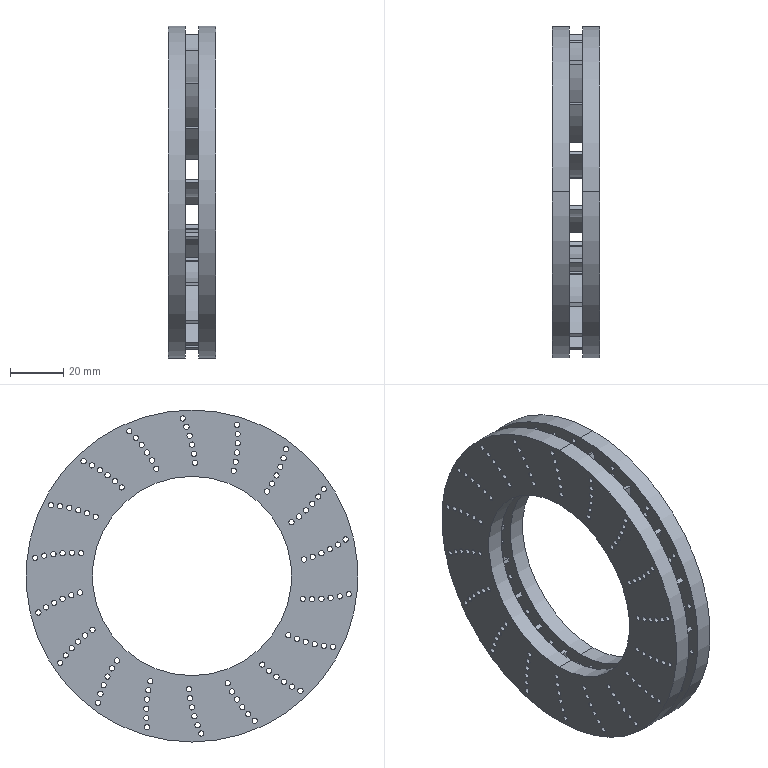Part | SolidWorks | features CirPattern 2, Fillet 2, ICE 2, BossThin 1, CurvePattern 1, Extrusion 1, MirrorPattern 1 | 1 solid | 522 faces | box 18 x 125 x 125 mm | volume 100342 mm3 | cylinder 484 | plane 38 | commonest cylinder face diameters 2 x432 60.048 x20 63.048 x20 1.5 x4 75 x4 125 x4